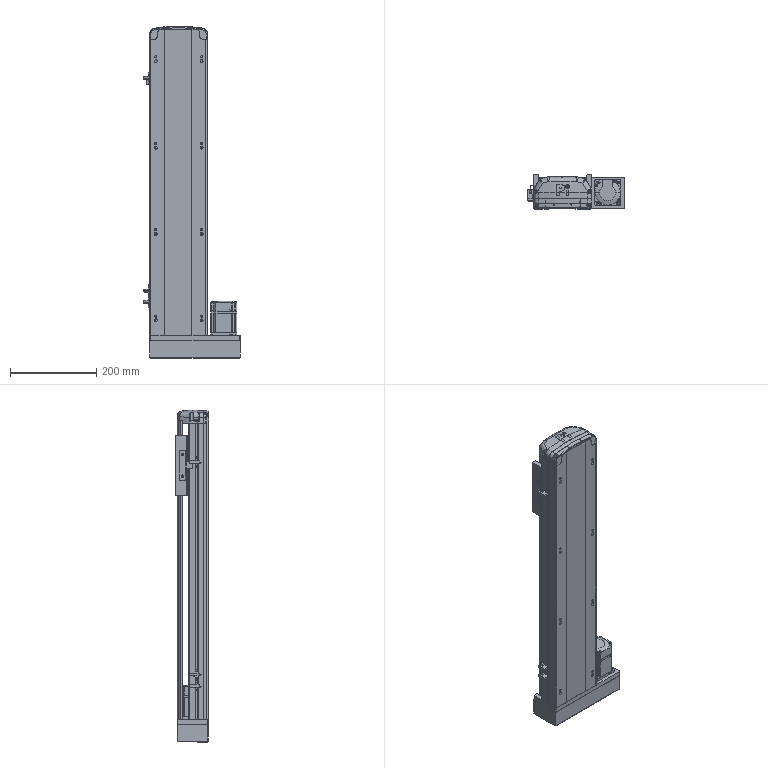Part | SolidWorks | features BaseBody 11 | 11 solids | 1770 faces | box 224 x 78.028 x 768.474 mm | volume 3697252 mm3 | plane 950 | cylinder 434 | spline 335 | cone 41 | torus 10 | commonest cylinder face diameters 4 x46 5 x40 8 x34 2 x29 0.6 x28 4.2 x20